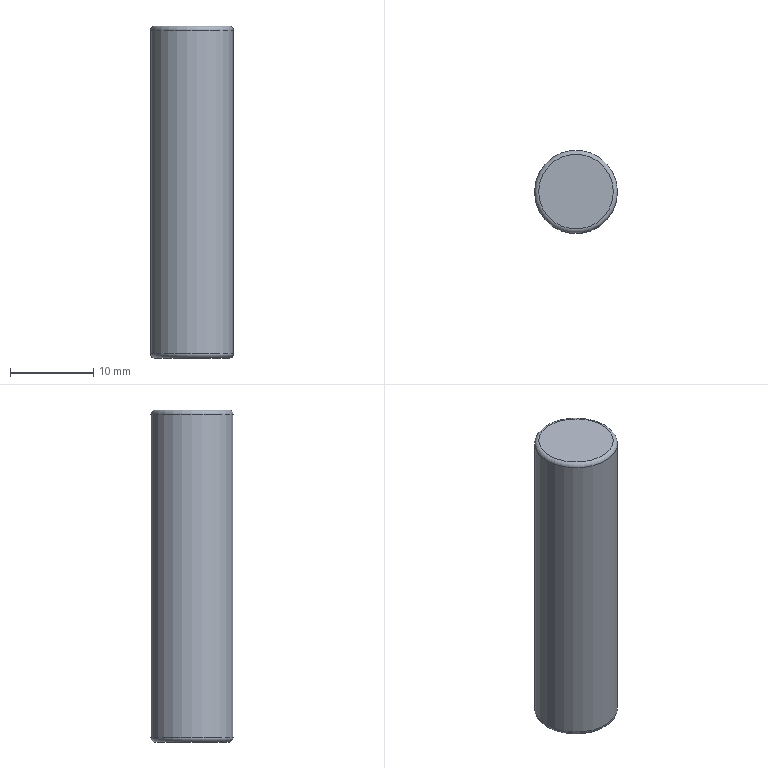Part | STEP file | solid 72 | 1 solid | 7 faces | box 10 x 10 x 40 mm | volume 2932 mm3 | cylinder 2 | plane 2 | torus 2 | cone 1 | commonest cylinder face diameters 5 x1 10 x1